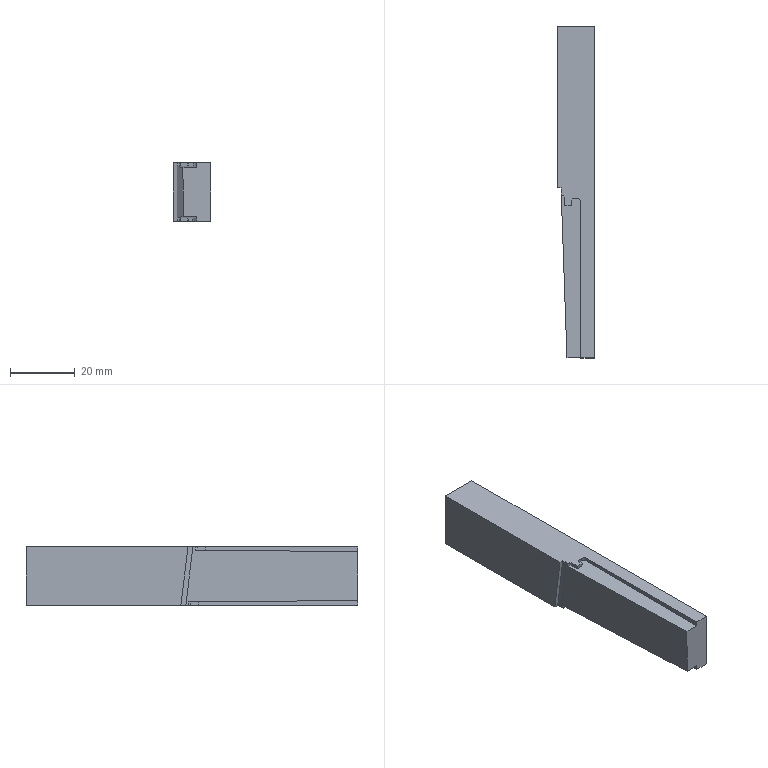Part | STEP file | 1 solid | 29 faces | box 11.534 x 102.36 x 18.001 mm | volume 18637 mm3 | plane 27 | cylinder 2 | commonest cylinder face diameters 2.01 x2